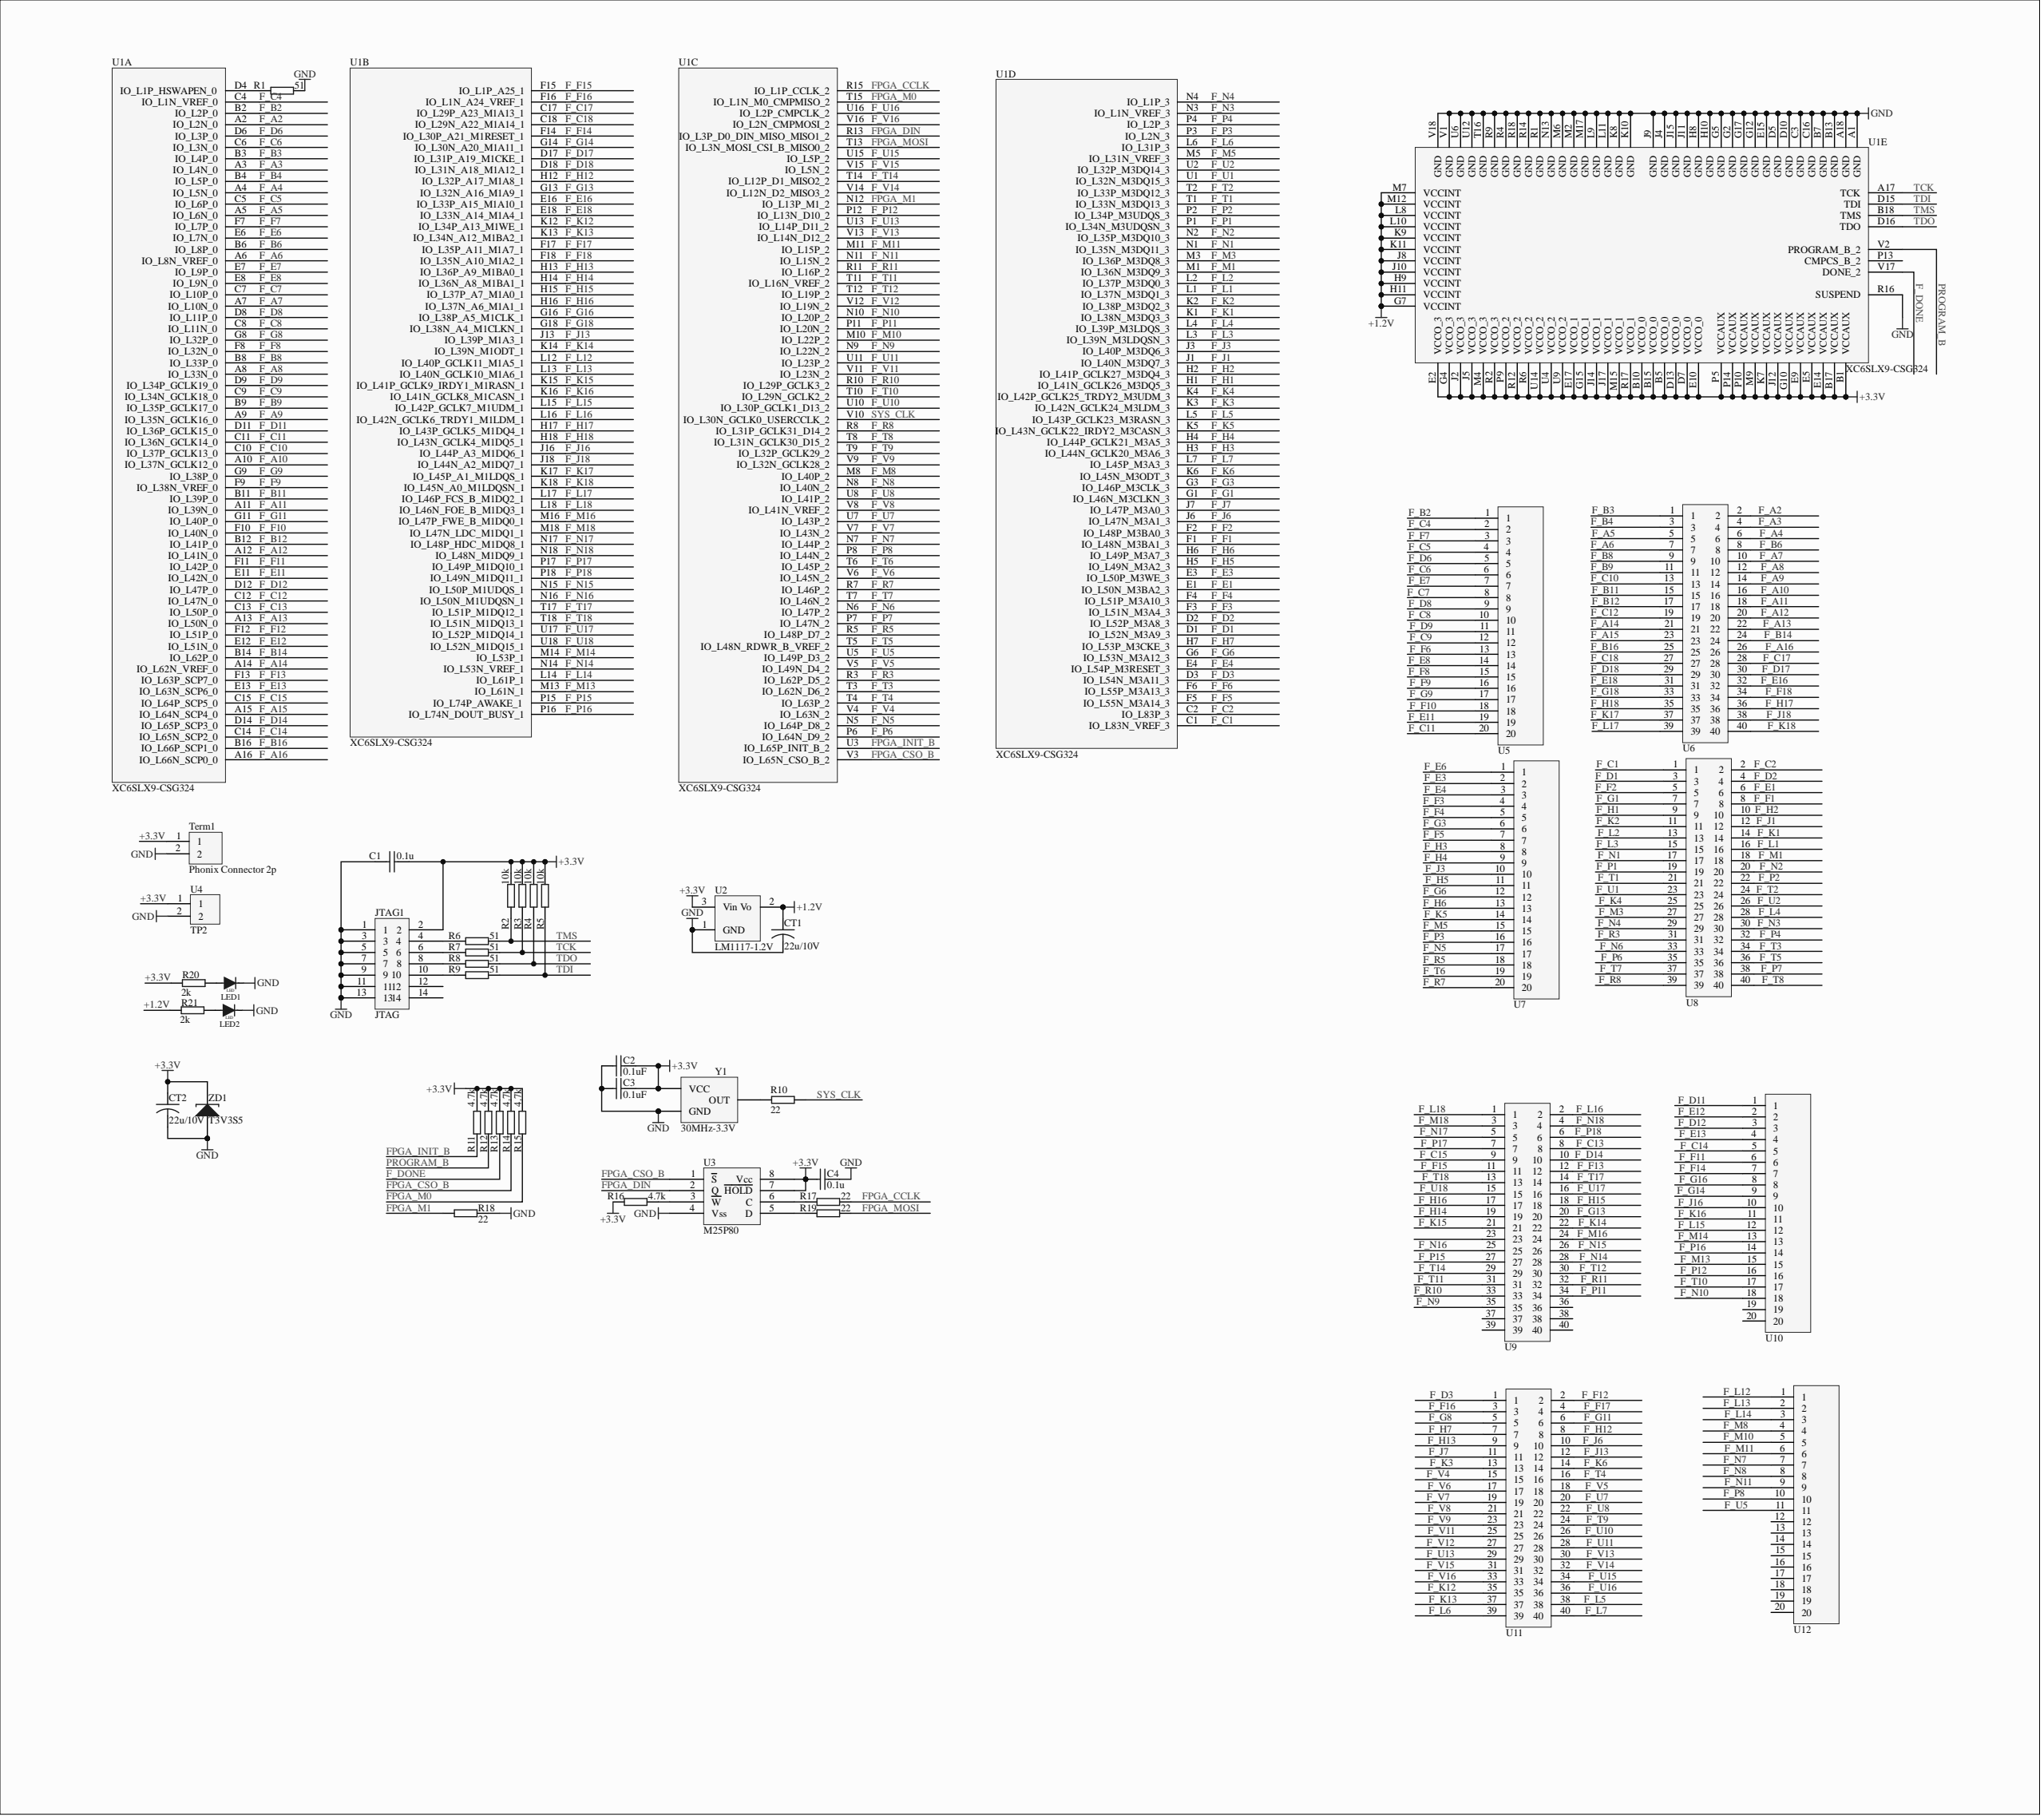Circuit board | Altium Designer | 45 parts | 251 nets
Bill of materials:
Comment,Description,Designator,Footprint,LibRef,Quantity
"0.1u","Multilayer ceramic capacitor","C1, C4","0603","CAP","2"
"0.1uF","Capacitor","C2, C3","0603","CAP","2"
"22u/10V","Capacitor","CT1, CT2","7227","CAPACITOR","2"
"JTAG","","JTAG1","IDC14S","IDC14","1"
"LED","","LED1, LED2","DIODE_2","LED","2"
"51","","R1, R6, R7, R8, R9","0603","RES2","5"
"10k","","R2, R3, R4, R5","0603","RES2","4"
"22","","R10, R17, R18, R19","0603","RES2","4"
"4.7k","","R11, R12, R13, R14, R15, R16","0603","RES2","6"
"2k","","R20, R21","0603","RES2","2"
"Phonix Connector 2p","Phonix Connector 2p","Term1","PhonixCon2P","Phonix Connector 2p","1"
"XC6SLX9-CSG324","","U1","CSG324","XC6SLX25-CSG324","1"
"LM1117-1.2V","","U2","SOT223","7810","1"
"M25P80","M25P80","U3","M25P16_SO-8","M25P80","1"
"TP2","TP2","U4","TP2","TP2","1"
"TP20_2.54mm","TP20_2.54mm","U5, U7, U10, U12","TP20_2.54mm","TP20_2.54mm","4"
"TP20*2_2.54mm","TP20*2_2.54mm","U6, U8, U9, U11","TP20*2_2.54mm","TP20*2_2.54mm","4"
"30MHz-3.3V","","Y1","OSC-SO4","OSCILLATOR","1"
"T3V3S5","Tunnel Diode - Dependent Source Model","ZD1","0603","D Tunnel2","1"
Netlist (Protel format):
[
C1
0603
0.1u



]
[
C2
0603
0.1uF



]
[
C3
0603
0.1uF



]
[
C4
0603
0.1u



]
[
CT1
7227
22u/10V



]
[
CT2
7227
22u/10V



]
[
JTAG1
IDC14S
JTAG



]
[
LED1
DIODE_2
LED



]
[
LED2
DIODE_2
LED



]
[
R1
0603
51



]
[
R2
0603
10k



]
[
R3
0603
10k



]
[
R4
0603
10k



]
[
R5
0603
10k



]
[
R6
0603
51



]
[
R7
0603
51



]
[
R8
0603
51



]
[
R9
0603
51



]
[
R10
0603
22



]
[
R11
0603
4.7k



]
[
R12
0603
4.7k



]
[
R13
0603
4.7k



]
[
R14
0603
4.7k



]
[
R15
0603
4.7k



]
[
R16
0603
4.7k



]
[
R17
0603
22



]
[
R18
0603
22



]
[
R19
0603
22



]
[
R20
0603
2k



]
[
R21
0603
2k



]
[
Term1
PhonixCon2P
Phonix Connector 2p



]
[
U1
CSG324
XC6SLX9-CSG324



]
[
U2
SOT223
LM1117-1.2V



]
[
U3
M25P16_SO-8
M25P80



]
[
U4
TP2
TP2



]
[
U5
TP20_2.54mm
TP20_2.54mm



]
[
U6
TP20*2_2.54mm
TP20*2_2.54mm



]
[
U7
TP20_2.54mm
TP20_2.54mm



]
[
U8
TP20*2_2.54mm
TP20*2_2.54mm



]
[
U9
TP20*2_2.54mm
TP20*2_2.54mm



]
[
U10
TP20_2.54mm
TP20_2.54mm



]
[
U11
TP20*2_2.54mm
TP20*2_2.54mm



]
[
U12
TP20_2.54mm
TP20_2.54mm



]
[
Y1
OSC-SO4
30MHz-3.3V



]
[
ZD1
0603
T3V3S5



]
(
TMS
R2-2
R6-1
U1-B18
)
(
TDO
R4-2
R8-1
U1-D16
)
(
TDI
R5-2
R9-1
U1-D15
)
(
TCK
R3-2
R7-1
U1-A17
)
(
SYS_CLK
R10-2
U1-V10
)
(
PROGRAM_B
R12-2
U1-V2
)
(
NetR19_2
R19-2
U3-5
)
(
NetR17_2
R17-2
U3-6
)
(
NetR16_1
R16-1
U3-3
)
(
NetR10_1
R10-1
Y1-3
)
(
NetR1_2
R1-2
U1-D4
)
(
NetLED2_A
LED2-A
R21-1
)
(
NetLED1_A
LED1-A
R20-1
)
(
NetJTAG1_10
JTAG1-10
R9-2
)
(
NetJTAG1_8
JTAG1-8
R8-2
)
(
NetJTAG1_6
JTAG1-6
R7-2
)
(
NetJTAG1_4
JTAG1-4
R6-2
)
(
GND
C1-1
C2-1
C3-1
C4-2
CT1-2
CT2-2
JTAG1-1
JTAG1-3
JTAG1-5
JTAG1-7
JTAG1-9
JTAG1-11
JTAG1-13
LED1-K
LED2-K
R1-1
R18-1
Term1-2
U1-A1
U1-A18
U1-B7
U1-B13
U1-C3
U1-C16
U1-D5
U1-D10
U1-E15
U1-G2
U1-G5
U1-G12
U1-G17
U1-H8
U1-H10
U1-J4
U1-J9
U1-J11
U1-J15
U1-K8
U1-K10
U1-L9
U1-L11
U1-M2
U1-M6
U1-M17
U1-N13
U1-R1
U1-R4
U1-R9
U1-R14
U1-R16
U1-R18
U1-T16
U1-U6
U1-U12
U1-V1
U1-V18
U2-1
U3-4
U4-2
Y1-2
ZD1-1
)
(
FPGA_MOSI
R19-1
U1-T13
)
(
FPGA_M1
R18-2
U1-N12
)
(
FPGA_M0
R15-2
U1-T15
)
(
FPGA_INIT_B
R11-2
U1-U3
)
(
FPGA_DIN
U1-R13
U3-2
)
(
FPGA_CSO_B
R14-2
U1-V3
U3-1
)
(
FPGA_CCLK
R17-1
U1-R15
)
(
F_V16
U1-V16
U11-33
)
(
F_V15
U1-V15
U11-31
)
(
F_V14
U1-V14
U11-32
)
(
F_V13
U1-V13
U11-30
)
(
F_V12
U1-V12
U11-27
)
(
F_V11
U1-V11
U11-25
)
(
F_V9
U1-V9
U11-23
)
(
F_V8
U1-V8
U11-21
)
(
F_V7
U1-V7
U11-19
)
(
F_V6
U1-V6
U11-17
)
(
F_V5
U1-V5
U11-18
)
(
F_V4
U1-V4
U11-15
)
(
F_U18
U1-U18
U9-15
)
(
F_U17
U1-U17
U9-16
)
(
F_U16
U1-U16
U11-36
)
(
F_U15
U1-U15
U11-34
)
(
F_U13
U1-U13
U11-29
)
(
F_U11
U1-U11
U11-28
)
(
F_U10
U1-U10
U11-26
)
(
F_U8
U1-U8
U11-22
)
(
F_U7
U1-U7
U11-20
)
(
F_U5
U1-U5
U12-11
)
(
F_U2
U1-U2
U8-26
)
(
F_U1
U1-U1
U8-23
)
(
F_T18
U1-T18
U9-13
)
(
F_T17
U1-T17
U9-14
)
(
F_T14
U1-T14
U9-29
)
(
F_T12
U1-T12
U9-30
)
(
F_T11
U1-T11
U9-31
)
(
F_T10
U1-T10
U10-17
)
(
F_T9
U1-T9
U11-24
)
(
F_T8
U1-T8
U8-40
)
(
F_T7
U1-T7
U8-37
)
(
F_T6
U1-T6
U7-19
)
(
F_T5
U1-T5
U8-36
)
(
F_T4
U1-T4
U11-16
)
(
F_T3
U1-T3
U8-34
)
(
F_T2
U1-T2
U8-24
)
(
F_T1
U1-T1
U8-21
)
(
F_R11
U1-R11
U9-32
)
(
F_R10
U1-R10
U9-33
)
(
F_R8
U1-R8
U8-39
)
(
F_R7
U1-R7
U7-20
)
(
F_R5
U1-R5
U7-18
)
(
F_R3
U1-R3
U8-31
)
(
F_P18
U1-P18
U9-6
)
(
F_P17
U1-P17
U9-7
)
(
F_P16
U1-P16
U10-14
)
(
F_P15
U1-P15
U9-27
)
(
F_P12
U1-P12
U10-16
)
(
F_P11
U1-P11
U9-34
)
(
F_P8
U1-P8
U12-10
)
(
F_P7
U1-P7
U8-38
)
(
F_P6
U1-P6
U8-35
)
(
F_P4
U1-P4
U8-32
)
(
F_P3
U1-P3
U7-16
)
(
F_P2
U1-P2
U8-22
)
(
F_P1
U1-P1
U8-19
)
(
F_N18
U1-N18
U9-4
)
(
F_N17
U1-N17
U9-5
)
(
F_N16
U1-N16
U9-25
)
(
F_N15
U1-N15
U9-26
)
(
F_N14
U1-N14
U9-28
)
(
F_N11
U1-N11
U12-9
)
(
F_N10
U1-N10
U10-18
)
(
F_N9
U1-N9
U9-35
)
(
F_N8
U1-N8
U12-8
)
(
F_N7
U1-N7
U12-7
)
(
F_N6
U1-N6
U8-33
)
(
F_N5
U1-N5
U7-17
)
(
F_N4
U1-N4
U8-29
)
(
F_N3
U1-N3
U8-30
)
(
F_N2
U1-N2
U8-20
)
(
F_N1
U1-N1
U8-17
)
(
F_M18
U1-M18
U9-3
)
(
F_M16
U1-M16
U9-24
)
(
F_M14
U1-M14
U10-13
)
(
F_M13
U1-M13
U10-15
)
(
F_M11
U1-M11
U12-6
)
(
F_M10
U1-M10
U12-5
)
(
F_M8
U1-M8
U12-4
)
(
F_M5
U1-M5
U7-15
)
(
F_M3
U1-M3
U8-27
)
(
F_M1
U1-M1
U8-18
)
(
F_L18
U1-L18
U9-1
)
(
F_L17
U1-L17
U6-39
)
(
F_L16
U1-L16
U9-2
)
(
F_L15
U1-L15
U10-12
)
(
F_L14
U1-L14
U12-3
)
(
F_L13
U1-L13
U12-2
)
(
F_L12
U1-L12
U12-1
)
(
F_L7
U1-L7
U11-40
)
(
F_L6
U1-L6
U11-39
)
(
F_L5
U1-L5
U11-38
)
(
F_L4
U1-L4
U8-28
)
(
F_L3
U1-L3
U8-15
)
(
F_L2
U1-L2
U8-13
)
(
F_L1
U1-L1
U8-16
)
(
F_K18
U1-K18
U6-40
)
(
F_K17
U1-K17
U6-37
)
(
F_K16
U1-K16
U10-11
)
(
F_K15
U1-K15
U9-21
)
(
F_K14
U1-K14
U9-22
)
(
F_K13
U1-K13
U11-37
)
(
F_K12
U1-K12
U11-35
)
(
F_K6
U1-K6
U11-14
)
(
F_K5
U1-K5
U7-14
)
(
F_K4
U1-K4
U8-25
)
(
F_K3
U1-K3
U11-13
)
(
F_K2
U1-K2
U8-11
)
(
F_K1
U1-K1
U8-14
)
(
F_J18
U1-J18
U6-38
)
(
F_J16
U1-J16
U10-10
)
(
F_J13
U1-J13
U11-12
)
(
F_J7
U1-J7
U11-11
)
(
F_J6
U1-J6
U11-10
)
(
F_J3
U1-J3
U7-10
)
(
F_J1
U1-J1
U8-12
)
(
F_H18
U1-H18
U6-35
)
(
F_H17
U1-H17
U6-36
)
(
F_H16
U1-H16
U9-17
)
(
F_H15
U1-H15
U9-18
)
(
F_H14
U1-H14
U9-19
)
(
F_H13
U1-H13
U11-9
)
(
F_H12
U1-H12
U11-8
)
(
F_H7
U1-H7
U11-7
)
(
F_H6
U1-H6
U7-13
)
(
F_H5
U1-H5
U7-11
)
(
F_H4
U1-H4
U7-9
)
(
F_H3
U1-H3
U7-8
)
(
F_H2
U1-H2
U8-10
)
(
F_H1
U1-H1
U8-9
)
(
F_G18
U1-G18
U6-33
)
(
F_G16
U1-G16
U10-8
)
(
F_G14
U1-G14
U10-9
)
(
F_G13
U1-G13
U9-20
)
(
F_G11
U1-G11
U11-6
)
(
F_G9
U1-G9
U5-17
)
(
F_G8
U1-G8
U11-5
)
(
F_G6
U1-G6
U7-12
)
(
F_G3
U1-G3
U7-6
)
(
F_G1
U1-G1
U8-7
)
(
F_F18
U1-F18
U6-34
)
(
F_F17
U1-F17
U11-4
)
(
F_F16
U1-F16
U11-3
)
(
F_F15
U1-F15
U9-11
)
(
F_F14
U1-F14
U10-7
)
(
F_F13
U1-F13
U9-12
)
(
F_F12
U1-F12
U11-2
)
(
F_F11
U1-F11
U10-6
)
(
F_F10
U1-F10
U5-18
)
(
F_F9
U1-F9
U5-16
)
(
F_F8
U1-F8
U5-15
)
(
F_F7
U1-F7
U5-3
)
(
F_F6
U1-F6
U5-13
)
(
F_F5
U1-F5
U7-7
)
(
F_F4
U1-F4
U7-5
)
(
F_F3
U1-F3
U7-4
)
(
F_F2
U1-F2
U8-5
)
(
F_F1
U1-F1
U8-8
)
(
F_E18
U1-E18
U6-31
)
(
F_E16
U1-E16
U6-32
)
(
F_E13
U1-E13
U10-4
)
(
F_E12
U1-E12
U10-2
)
(
F_E11
U1-E11
U5-19
)
(
F_E8
U1-E8
U5-14
)
(
F_E7
U1-E7
U5-7
)
(
F_E6
U1-E6
U7-1
)
(
F_E4
U1-E4
U7-3
)
(
F_E3
U1-E3
U7-2
)
(
F_E1
U1-E1
U8-6
)
(
F_DONE
R13-2
U1-V17
)
(
F_D18
U1-D18
U6-29
)
(
F_D17
U1-D17
U6-30
)
(
F_D14
U1-D14
U9-10
)
(
F_D12
U1-D12
U10-3
)
(
F_D11
U1-D11
U10-1
)
(
F_D9
U1-D9
U5-11
)
(
F_D8
U1-D8
U5-9
)
(
F_D6
U1-D6
U5-5
)
(
F_D3
U1-D3
U11-1
)
(
F_D2
U1-D2
U8-4
)
(
F_D1
U1-D1
U8-3
)
(
F_C18
U1-C18
U6-27
)
(
F_C17
U1-C17
U6-28
)
(
F_C15
U1-C15
U9-9
)
(
F_C14
U1-C14
U10-5
)
(
F_C13
U1-C13
U9-8
)
(
F_C12
U1-C12
U6-19
)
(
F_C11
U1-C11
U5-20
)
(
F_C10
U1-C10
U6-13
)
(
F_C9
U1-C9
U5-12
)
(
F_C8
U1-C8
U5-10
)
(
F_C7
U1-C7
U5-8
)
(
F_C6
U1-C6
U5-6
)
(
F_C5
U1-C5
U5-4
)
(
F_C4
U1-C4
U5-2
)
(
F_C2
U1-C2
U8-2
)
(
F_C1
U1-C1
U8-1
)
(
F_B16
U1-B16
U6-25
)
(
F_B14
U1-B14
U6-24
)
(
F_B12
U1-B12
U6-17
)
(
F_B11
U1-B11
U6-15
)
(
F_B9
U1-B9
U6-11
)
(
F_B8
U1-B8
U6-9
)
(
F_B6
U1-B6
U6-8
)
(
F_B4
U1-B4
U6-3
)
(
F_B3
U1-B3
U6-1
)
(
F_B2
U1-B2
U5-1
)
(
F_A16
U1-A16
U6-26
)
(
F_A15
U1-A15
U6-23
)
(
F_A14
U1-A14
U6-21
)
(
F_A13
U1-A13
U6-22
)
(
F_A12
U1-A12
U6-20
)
(
F_A11
U1-A11
U6-18
)
(
F_A10
U1-A10
U6-16
)
(
F_A9
U1-A9
U6-14
)
(
F_A8
U1-A8
U6-12
)
(
F_A7
U1-A7
U6-10
)
(
F_A6
U1-A6
U6-7
)
(
F_A5
U1-A5
U6-5
)
(
F_A4
U1-A4
U6-6
)
(
F_A3
U1-A3
U6-4
)
(
F_A2
U1-A2
U6-2
)
(
+3.3V
C1-2
C2-2
C3-2
C4-1
CT2-1
JTAG1-2
R2-1
R3-1
R4-1
R5-1
R11-1
R12-1
R13-1
R14-1
R15-1
R16-2
R20-2
Term1-1
U1-B1
U1-B5
U1-B10
U1-B15
U1-B17
U1-D7
U1-D13
U1-E2
U1-E5
U1-E9
U1-E10
U1-E14
U1-E17
U1-G4
U1-G10
U1-G15
U1-J2
U1-J5
U1-J12
U1-J14
U1-J17
U1-K7
U1-M4
U1-M9
U1-M15
U1-P5
U1-P9
U1-P10
U1-P14
U1-R2
U1-R6
U1-R12
U1-R17
U1-U4
U1-U9
U1-U14
U2-3
U3-7
U3-8
U4-1
Y1-4
ZD1-2
)
(
+1.2V
CT1-1
R21-2
U1-G7
U1-H9
U1-H11
U1-J8
U1-J10
U1-K9
U1-K11
U1-L8
U1-L10
U1-M7
U1-M12
U2-2
)